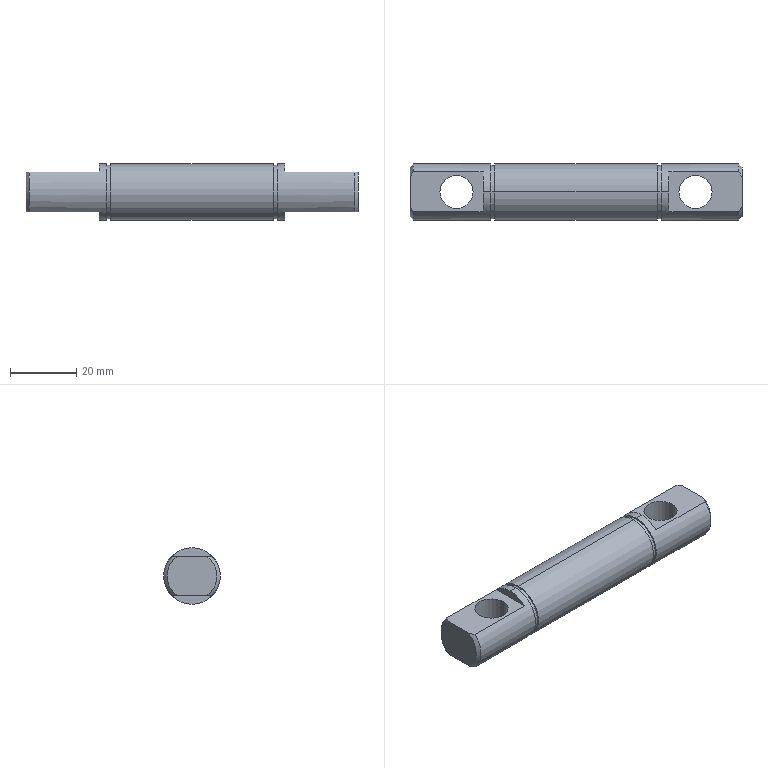Part | STEP file | tension shaft 2_SUS304 | 1 solid | 32 faces | box 100 x 17 x 17 mm | volume 18904 mm3 | cylinder 14 | plane 14 | cone 4 | commonest cylinder face diameters 17 x6 10 x4 16.1 x4